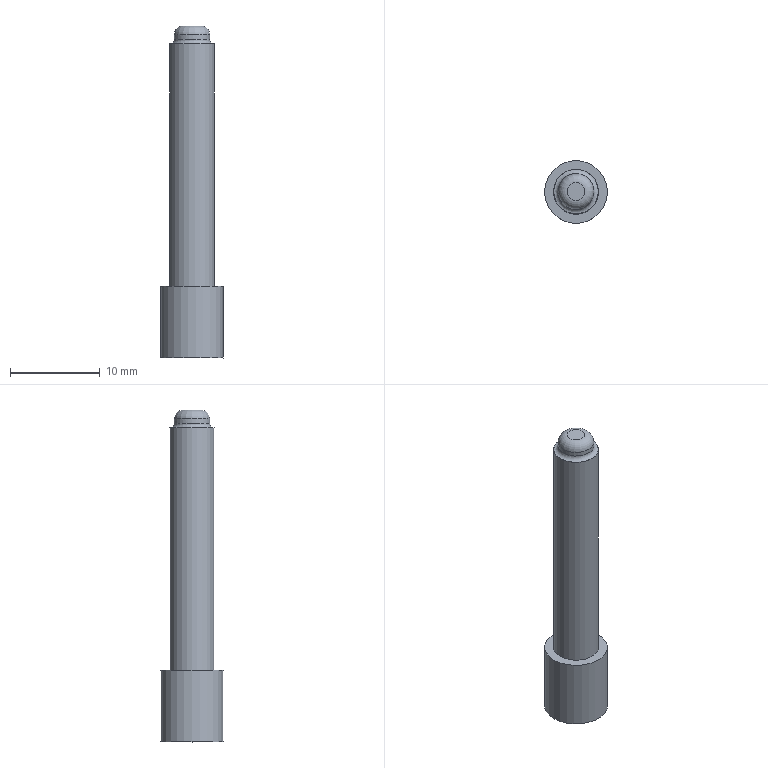Part | NX | features solid 2 | 1 solid | 9 faces | box 7 x 7 x 37 mm | volume 861.228 mm3 | plane 4 | cylinder 3 | torus 2 | commonest cylinder face diameters 3.98 x1 5 x1 7 x1
STEP:
#1=CARTESIAN_POINT('',(4211.736,-839.122,858.716));
#2=VERTEX_POINT('',#1);
#3=CARTESIAN_POINT('',(4209.236,-839.122,858.716));
#4=DIRECTION('',(0.,0.,1.));
#5=DIRECTION('',(1.,0.,0.));
#6=AXIS2_PLACEMENT_3D('',#3,#4,#5);
#7=CIRCLE('',#6,2.5);
#8=EDGE_CURVE('',#2,#2,#7,.T.);
#9=ORIENTED_EDGE('',*,*,#8,.F.);
#10=EDGE_LOOP('',(#9));
#11=FACE_BOUND('',#10,.T.);
#12=CARTESIAN_POINT('',(4206.736,-839.122,831.716));
#13=VERTEX_POINT('',#12);
#14=CARTESIAN_POINT('',(4209.236,-839.122,831.716));
#15=DIRECTION('',(0.,0.,-1.));
#16=DIRECTION('',(-1.,0.,0.));
#17=AXIS2_PLACEMENT_3D('',#14,#15,#16);
#18=CIRCLE('',#17,2.5);
#19=EDGE_CURVE('',#13,#13,#18,.F.);
#20=ORIENTED_EDGE('',*,*,#19,.T.);
#21=EDGE_LOOP('',(#20));
#22=FACE_BOUND('',#21,.T.);
#23=CARTESIAN_POINT('',(4209.236,-839.122,823.716));
#24=DIRECTION('',(0.,0.,1.));
#25=DIRECTION('',(1.,0.,0.));
#26=AXIS2_PLACEMENT_3D('',#23,#24,#25);
#27=CYLINDRICAL_SURFACE('',#26,2.5);
#28=ADVANCED_FACE('',(#11,#22),#27,.T.);
#29=CARTESIAN_POINT('',(4207.29,-839.538,859.716));
#30=VERTEX_POINT('',#29);
#31=CARTESIAN_POINT('',(4208.039,-840.975,859.716));
#32=CARTESIAN_POINT('',(4207.079,-839.583,859.716));
#33=CARTESIAN_POINT('',(4207.386,-837.923,859.716));
#34=CARTESIAN_POINT('',(4208.774,-836.966,859.716));
#35=CARTESIAN_POINT('',(4210.434,-837.27,859.716));
#36=CARTESIAN_POINT('',(4211.392,-838.661,859.716));
#37=CARTESIAN_POINT('',(4211.088,-840.319,859.716));
#38=CARTESIAN_POINT('',(4209.699,-841.278,859.716));
#39=CARTESIAN_POINT('',(4208.039,-840.975,859.716));
#40=CARTESIAN_POINT('',(4207.079,-839.583,859.716));
#41=CARTESIAN_POINT('',(4207.386,-837.923,859.716));
#42=B_SPLINE_CURVE_WITH_KNOTS('',3,(#31,#32,#33,#34,#35,#36,#37,#38,#39,#40,#41),.UNSPECIFIED.,.T.,.F.,(1,1,1,1,1,1,1,1,1,1,1,1,1,1,1),(-0.004666,-0.00311,-0.001555,0.,0.001555,0.00311,0.004666,0.006221,0.007776,0.009331,0.01089,0.01244,0.014,0.01555,0.01711),.UNSPECIFIED.);
#43=EDGE_CURVE('',#30,#30,#42,.T.);
#44=ORIENTED_EDGE('',*,*,#43,.T.);
#45=EDGE_LOOP('',(#44));
#46=FACE_BOUND('',#45,.T.);
#47=CARTESIAN_POINT('',(4211.226,-839.122,859.216));
#48=VERTEX_POINT('',#47);
#49=CARTESIAN_POINT('',(4209.236,-839.122,859.216));
#50=DIRECTION('',(0.,0.,1.));
#51=DIRECTION('',(1.,0.,0.));
#52=AXIS2_PLACEMENT_3D('',#49,#50,#51);
#53=CIRCLE('',#52,1.99);
#54=EDGE_CURVE('',#48,#48,#53,.F.);
#55=ORIENTED_EDGE('',*,*,#54,.F.);
#56=EDGE_LOOP('',(#55));
#57=FACE_BOUND('',#56,.T.);
#58=CARTESIAN_POINT('',(4209.236,-839.122,860.716));
#59=DIRECTION('',(0.,0.,-1.));
#60=DIRECTION('',(-1.,0.,0.));
#61=AXIS2_PLACEMENT_3D('',#58,#59,#60);
#62=CYLINDRICAL_SURFACE('',#61,1.99);
#63=ADVANCED_FACE('',(#46,#57),#62,.T.);
#64=CARTESIAN_POINT('',(4208.246,-839.122,860.716));
#65=VERTEX_POINT('',#64);
#66=CARTESIAN_POINT('',(4209.236,-839.122,860.716));
#67=DIRECTION('',(0.,0.,-1.));
#68=DIRECTION('',(-1.,0.,0.));
#69=AXIS2_PLACEMENT_3D('',#66,#67,#68);
#70=CIRCLE('',#69,0.99);
#71=EDGE_CURVE('',#65,#65,#70,.F.);
#72=ORIENTED_EDGE('',*,*,#71,.T.);
#73=EDGE_LOOP('',(#72));
#74=FACE_BOUND('',#73,.T.);
#75=CARTESIAN_POINT('',(4209.236,-839.122,860.716));
#76=DIRECTION('',(0.,0.,-1.));
#77=DIRECTION('',(-1.,0.,0.));
#78=AXIS2_PLACEMENT_3D('',#75,#76,#77);
#79=PLANE('',#78);
#80=ADVANCED_FACE('',(#74),#79,.F.);
#81=CARTESIAN_POINT('',(4211.726,-839.122,858.716));
#82=VERTEX_POINT('',#81);
#83=CARTESIAN_POINT('',(4209.236,-839.122,858.716));
#84=DIRECTION('',(0.,0.,1.));
#85=DIRECTION('',(1.,0.,0.));
#86=AXIS2_PLACEMENT_3D('',#83,#84,#85);
#87=CIRCLE('',#86,2.49);
#88=EDGE_CURVE('',#82,#82,#87,.F.);
#89=ORIENTED_EDGE('',*,*,#88,.F.);
#90=EDGE_LOOP('',(#89));
#91=FACE_BOUND('',#90,.T.);
#92=ORIENTED_EDGE('',*,*,#54,.T.);
#93=EDGE_LOOP('',(#92));
#94=FACE_BOUND('',#93,.T.);
#95=CARTESIAN_POINT('',(4209.236,-839.122,859.216));
#96=DIRECTION('',(0.,0.,1.));
#97=DIRECTION('',(1.,0.,0.));
#98=AXIS2_PLACEMENT_3D('',#95,#96,#97);
#99=TOROIDAL_SURFACE('',#98,2.49,0.5);
#100=ADVANCED_FACE('',(#91,#94),#99,.F.);
#101=ORIENTED_EDGE('',*,*,#88,.T.);
#102=EDGE_LOOP('',(#101));
#103=FACE_BOUND('',#102,.T.);
#104=ORIENTED_EDGE('',*,*,#8,.T.);
#105=EDGE_LOOP('',(#104));
#106=FACE_BOUND('',#105,.T.);
#107=CARTESIAN_POINT('',(4217.236,-839.122,858.716));
#108=DIRECTION('',(0.,0.,1.));
#109=DIRECTION('',(1.,0.,0.));
#110=AXIS2_PLACEMENT_3D('',#107,#108,#109);
#111=PLANE('',#110);
#112=ADVANCED_FACE('',(#103,#106),#111,.T.);
#113=ORIENTED_EDGE('',*,*,#71,.F.);
#114=EDGE_LOOP('',(#113));
#115=FACE_BOUND('',#114,.T.);
#116=ORIENTED_EDGE('',*,*,#43,.F.);
#117=EDGE_LOOP('',(#116));
#118=FACE_BOUND('',#117,.T.);
#119=CARTESIAN_POINT('',(4209.236,-839.122,859.716));
#120=DIRECTION('',(0.,0.,-1.));
#121=DIRECTION('',(-1.,0.,0.));
#122=AXIS2_PLACEMENT_3D('',#119,#120,#121);
#123=DEGENERATE_TOROIDAL_SURFACE('',#122,0.99,1.,.T.);
#124=ADVANCED_FACE('',(#115,#118),#123,.T.);
#125=CARTESIAN_POINT('',(4205.736,-839.122,823.716));
#126=VERTEX_POINT('',#125);
#127=CARTESIAN_POINT('',(4209.236,-839.122,823.716));
#128=DIRECTION('',(0.,0.,-1.));
#129=DIRECTION('',(-1.,0.,0.));
#130=AXIS2_PLACEMENT_3D('',#127,#128,#129);
#131=CIRCLE('',#130,3.5);
#132=EDGE_CURVE('',#126,#126,#131,.T.);
#133=ORIENTED_EDGE('',*,*,#132,.T.);
#134=EDGE_LOOP('',(#133));
#135=FACE_BOUND('',#134,.T.);
#136=CARTESIAN_POINT('',(4209.236,-839.122,823.716));
#137=DIRECTION('',(0.,0.,-1.));
#138=DIRECTION('',(-1.,0.,0.));
#139=AXIS2_PLACEMENT_3D('',#136,#137,#138);
#140=PLANE('',#139);
#141=ADVANCED_FACE('',(#135),#140,.T.);
#142=CARTESIAN_POINT('',(4205.736,-839.122,831.716));
#143=VERTEX_POINT('',#142);
#144=CARTESIAN_POINT('',(4209.236,-839.122,831.716));
#145=DIRECTION('',(0.,0.,-1.));
#146=DIRECTION('',(-1.,0.,0.));
#147=AXIS2_PLACEMENT_3D('',#144,#145,#146);
#148=CIRCLE('',#147,3.5);
#149=EDGE_CURVE('',#143,#143,#148,.T.);
#150=ORIENTED_EDGE('',*,*,#149,.T.);
#151=EDGE_LOOP('',(#150));
#152=FACE_BOUND('',#151,.T.);
#153=ORIENTED_EDGE('',*,*,#132,.F.);
#154=EDGE_LOOP('',(#153));
#155=FACE_BOUND('',#154,.T.);
#156=CARTESIAN_POINT('',(4209.236,-839.122,823.716));
#157=DIRECTION('',(0.,0.,1.));
#158=DIRECTION('',(1.,0.,0.));
#159=AXIS2_PLACEMENT_3D('',#156,#157,#158);
#160=CYLINDRICAL_SURFACE('',#159,3.5);
#161=ADVANCED_FACE('',(#152,#155),#160,.T.);
#162=ORIENTED_EDGE('',*,*,#19,.F.);
#163=EDGE_LOOP('',(#162));
#164=FACE_BOUND('',#163,.T.);
#165=ORIENTED_EDGE('',*,*,#149,.F.);
#166=EDGE_LOOP('',(#165));
#167=FACE_BOUND('',#166,.T.);
#168=CARTESIAN_POINT('',(4217.236,-877.122,831.716));
#169=DIRECTION('',(0.,0.,-1.));
#170=DIRECTION('',(-1.,0.,0.));
#171=AXIS2_PLACEMENT_3D('',#168,#169,#170);
#172=PLANE('',#171);
#173=ADVANCED_FACE('',(#164,#167),#172,.F.);
#174=CLOSED_SHELL('',(#28,#63,#80,#100,#112,#124,#141,#161,#173));
#175=MANIFOLD_SOLID_BREP('',#174);
#176=(LENGTH_UNIT()NAMED_UNIT(*)SI_UNIT(.MILLI.,.METRE.));
#177=UNCERTAINTY_MEASURE_WITH_UNIT(LENGTH_MEASURE(0.0508),#176,'','');
#178=(NAMED_UNIT(*)PLANE_ANGLE_UNIT()SI_UNIT($,.RADIAN.));
#179=(NAMED_UNIT(*)SI_UNIT($,.STERADIAN.)SOLID_ANGLE_UNIT());
#180=(GEOMETRIC_REPRESENTATION_CONTEXT(3)GLOBAL_UNCERTAINTY_ASSIGNED_CONTEXT((#177))GLOBAL_UNIT_ASSIGNED_CONTEXT((#176,#178,#179))REPRESENTATION_CONTEXT('',''));
#181=ADVANCED_BREP_SHAPE_REPRESENTATION('',(#175),#180);